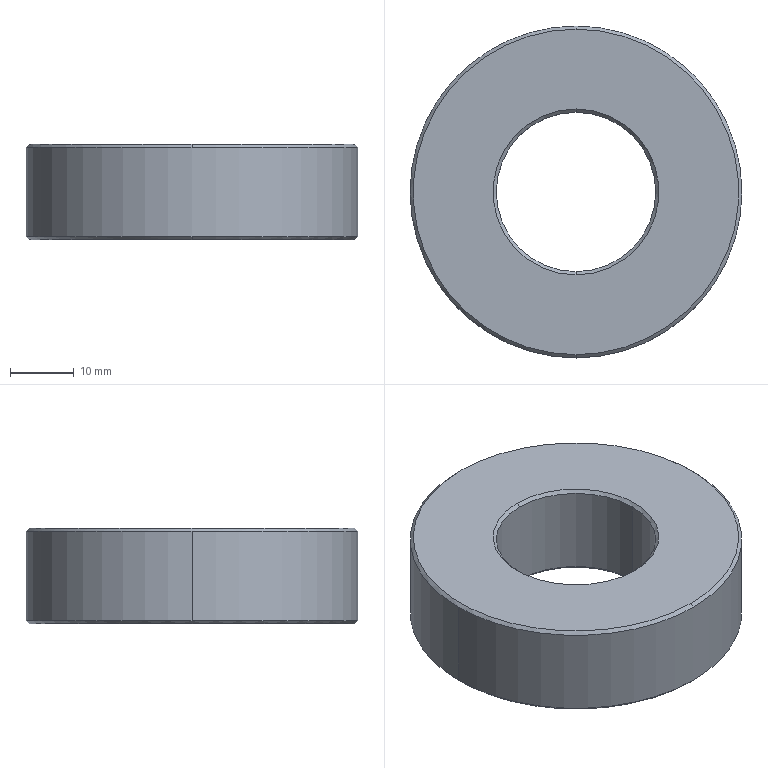Part | 1 solid | 14 faces | box 52 x 52 x 15 mm | volume 24432 mm3 | cone 8 | cylinder 4 | plane 2 | commonest cylinder face diameters 25 x2 52 x2
STEP:
#1=CARTESIAN_POINT('',(0.,-25.5,-7.5));
#2=VERTEX_POINT('',#1);
#3=CARTESIAN_POINT('',(0.,25.5,-7.5));
#4=VERTEX_POINT('',#3);
#5=CARTESIAN_POINT('',(0.,0.,-7.5));
#6=DIRECTION('',(0.,0.,1.));
#7=DIRECTION('',(0.,-1.,0.));
#8=AXIS2_PLACEMENT_3D('',#5,#6,#7);
#9=CIRCLE('',#8,25.5);
#10=EDGE_CURVE('',#2,#4,#9,.T.);
#11=ORIENTED_EDGE('',*,*,#10,.T.);
#12=CARTESIAN_POINT('',(0.,26.,-7.));
#13=VERTEX_POINT('',#12);
#14=CARTESIAN_POINT('',(0.,26.,-7.));
#15=DIRECTION('',(0.,0.7071,0.7071));
#16=VECTOR('',#15,1000.);
#17=LINE('',#14,#16);
#18=EDGE_CURVE('',#4,#13,#17,.T.);
#19=ORIENTED_EDGE('',*,*,#18,.T.);
#20=CARTESIAN_POINT('',(26.,0.,-7.));
#21=VERTEX_POINT('',#20);
#22=CARTESIAN_POINT('',(0.,0.,-7.));
#23=DIRECTION('',(0.,0.,-1.));
#24=DIRECTION('',(1.,0.,0.));
#25=AXIS2_PLACEMENT_3D('',#22,#23,#24);
#26=CIRCLE('',#25,26.);
#27=EDGE_CURVE('',#13,#21,#26,.T.);
#28=ORIENTED_EDGE('',*,*,#27,.T.);
#29=CARTESIAN_POINT('',(0.,-26.,-7.));
#30=VERTEX_POINT('',#29);
#31=CARTESIAN_POINT('',(0.,0.,-7.));
#32=DIRECTION('',(0.,0.,-1.));
#33=DIRECTION('',(1.,0.,0.));
#34=AXIS2_PLACEMENT_3D('',#31,#32,#33);
#35=CIRCLE('',#34,26.);
#36=EDGE_CURVE('',#21,#30,#35,.T.);
#37=ORIENTED_EDGE('',*,*,#36,.T.);
#38=CARTESIAN_POINT('',(0.,-26.,-7.));
#39=DIRECTION('',(0.,-0.7071,0.7071));
#40=VECTOR('',#39,1000.);
#41=LINE('',#38,#40);
#42=EDGE_CURVE('',#2,#30,#41,.T.);
#43=ORIENTED_EDGE('',*,*,#42,.F.);
#44=EDGE_LOOP('',(#11,#19,#28,#37,#43));
#45=FACE_OUTER_BOUND('',#44,.T.);
#46=CARTESIAN_POINT('',(0.,0.,-7.));
#47=DIRECTION('',(0.,0.,1.));
#48=DIRECTION('',(0.,-1.,0.));
#49=AXIS2_PLACEMENT_3D('',#46,#47,#48);
#50=CONICAL_SURFACE('',#49,26.,0.7854);
#51=ADVANCED_FACE('',(#45),#50,.T.);
#52=CARTESIAN_POINT('',(0.,-12.5,-7.));
#53=VERTEX_POINT('',#52);
#54=CARTESIAN_POINT('',(-12.5,0.,-7.));
#55=VERTEX_POINT('',#54);
#56=CARTESIAN_POINT('',(0.,0.,-7.));
#57=DIRECTION('',(0.,0.,-1.));
#58=DIRECTION('',(-1.,0.,0.));
#59=AXIS2_PLACEMENT_3D('',#56,#57,#58);
#60=CIRCLE('',#59,12.5);
#61=EDGE_CURVE('',#53,#55,#60,.T.);
#62=ORIENTED_EDGE('',*,*,#61,.F.);
#63=CARTESIAN_POINT('',(0.,-13.,-7.5));
#64=VERTEX_POINT('',#63);
#65=CARTESIAN_POINT('',(0.,-13.,-7.5));
#66=DIRECTION('',(0.,-0.7071,-0.7071));
#67=VECTOR('',#66,1000.);
#68=LINE('',#65,#67);
#69=EDGE_CURVE('',#53,#64,#68,.T.);
#70=ORIENTED_EDGE('',*,*,#69,.T.);
#71=CARTESIAN_POINT('',(0.,13.,-7.5));
#72=VERTEX_POINT('',#71);
#73=CARTESIAN_POINT('',(0.,0.,-7.5));
#74=DIRECTION('',(0.,0.,-1.));
#75=DIRECTION('',(0.,1.,0.));
#76=AXIS2_PLACEMENT_3D('',#73,#74,#75);
#77=CIRCLE('',#76,13.);
#78=EDGE_CURVE('',#64,#72,#77,.T.);
#79=ORIENTED_EDGE('',*,*,#78,.T.);
#80=CARTESIAN_POINT('',(0.,12.5,-7.));
#81=VERTEX_POINT('',#80);
#82=CARTESIAN_POINT('',(0.,13.,-7.5));
#83=DIRECTION('',(0.,0.7071,-0.7071));
#84=VECTOR('',#83,1000.);
#85=LINE('',#82,#84);
#86=EDGE_CURVE('',#81,#72,#85,.T.);
#87=ORIENTED_EDGE('',*,*,#86,.F.);
#88=CARTESIAN_POINT('',(0.,0.,-7.));
#89=DIRECTION('',(0.,0.,-1.));
#90=DIRECTION('',(-1.,0.,0.));
#91=AXIS2_PLACEMENT_3D('',#88,#89,#90);
#92=CIRCLE('',#91,12.5);
#93=EDGE_CURVE('',#55,#81,#92,.T.);
#94=ORIENTED_EDGE('',*,*,#93,.F.);
#95=EDGE_LOOP('',(#62,#70,#79,#87,#94));
#96=FACE_OUTER_BOUND('',#95,.T.);
#97=CARTESIAN_POINT('',(0.,0.,-7.5));
#98=DIRECTION('',(0.,0.,-1.));
#99=DIRECTION('',(0.,1.,0.));
#100=AXIS2_PLACEMENT_3D('',#97,#98,#99);
#101=CONICAL_SURFACE('',#100,13.,0.7854);
#102=ADVANCED_FACE('',(#96),#101,.F.);
#103=CARTESIAN_POINT('',(0.,26.,7.));
#104=VERTEX_POINT('',#103);
#105=CARTESIAN_POINT('',(26.,0.,7.));
#106=VERTEX_POINT('',#105);
#107=CARTESIAN_POINT('',(0.,0.,7.));
#108=DIRECTION('',(0.,0.,-1.));
#109=DIRECTION('',(-1.,0.,0.));
#110=AXIS2_PLACEMENT_3D('',#107,#108,#109);
#111=CIRCLE('',#110,26.);
#112=EDGE_CURVE('',#104,#106,#111,.T.);
#113=ORIENTED_EDGE('',*,*,#112,.T.);
#114=CARTESIAN_POINT('',(26.,0.,7.5));
#115=DIRECTION('',(0.,0.,-1.));
#116=VECTOR('',#115,1000.);
#117=LINE('',#114,#116);
#118=EDGE_CURVE('',#106,#21,#117,.T.);
#119=ORIENTED_EDGE('',*,*,#118,.T.);
#120=ORIENTED_EDGE('',*,*,#27,.F.);
#121=CARTESIAN_POINT('',(-26.,0.,-7.));
#122=VERTEX_POINT('',#121);
#123=CARTESIAN_POINT('',(0.,0.,-7.));
#124=DIRECTION('',(0.,0.,-1.));
#125=DIRECTION('',(1.,0.,0.));
#126=AXIS2_PLACEMENT_3D('',#123,#124,#125);
#127=CIRCLE('',#126,26.);
#128=EDGE_CURVE('',#122,#13,#127,.T.);
#129=ORIENTED_EDGE('',*,*,#128,.F.);
#130=CARTESIAN_POINT('',(-26.,0.,7.));
#131=VERTEX_POINT('',#130);
#132=CARTESIAN_POINT('',(-26.,0.,7.5));
#133=DIRECTION('',(0.,0.,-1.));
#134=VECTOR('',#133,1000.);
#135=LINE('',#132,#134);
#136=EDGE_CURVE('',#131,#122,#135,.T.);
#137=ORIENTED_EDGE('',*,*,#136,.F.);
#138=CARTESIAN_POINT('',(0.,0.,7.));
#139=DIRECTION('',(0.,0.,-1.));
#140=DIRECTION('',(-1.,0.,0.));
#141=AXIS2_PLACEMENT_3D('',#138,#139,#140);
#142=CIRCLE('',#141,26.);
#143=EDGE_CURVE('',#131,#104,#142,.T.);
#144=ORIENTED_EDGE('',*,*,#143,.T.);
#145=EDGE_LOOP('',(#113,#119,#120,#129,#137,#144));
#146=FACE_OUTER_BOUND('',#145,.T.);
#147=CARTESIAN_POINT('',(0.,0.,7.5));
#148=DIRECTION('',(0.,0.,-1.));
#149=DIRECTION('',(-1.,0.,0.));
#150=AXIS2_PLACEMENT_3D('',#147,#148,#149);
#151=CYLINDRICAL_SURFACE('',#150,26.);
#152=ADVANCED_FACE('',(#146),#151,.T.);
#153=CARTESIAN_POINT('',(12.5,0.,7.));
#154=VERTEX_POINT('',#153);
#155=CARTESIAN_POINT('',(0.,-12.5,7.));
#156=VERTEX_POINT('',#155);
#157=CARTESIAN_POINT('',(0.,0.,7.));
#158=DIRECTION('',(0.,0.,-1.));
#159=DIRECTION('',(-1.,0.,0.));
#160=AXIS2_PLACEMENT_3D('',#157,#158,#159);
#161=CIRCLE('',#160,12.5);
#162=EDGE_CURVE('',#154,#156,#161,.T.);
#163=ORIENTED_EDGE('',*,*,#162,.F.);
#164=CARTESIAN_POINT('',(12.5,0.,-7.));
#165=VERTEX_POINT('',#164);
#166=CARTESIAN_POINT('',(12.5,0.,7.5));
#167=DIRECTION('',(0.,0.,-1.));
#168=VECTOR('',#167,1000.);
#169=LINE('',#166,#168);
#170=EDGE_CURVE('',#154,#165,#169,.T.);
#171=ORIENTED_EDGE('',*,*,#170,.T.);
#172=CARTESIAN_POINT('',(0.,0.,-7.));
#173=DIRECTION('',(0.,0.,-1.));
#174=DIRECTION('',(-1.,0.,0.));
#175=AXIS2_PLACEMENT_3D('',#172,#173,#174);
#176=CIRCLE('',#175,12.5);
#177=EDGE_CURVE('',#165,#53,#176,.T.);
#178=ORIENTED_EDGE('',*,*,#177,.T.);
#179=ORIENTED_EDGE('',*,*,#61,.T.);
#180=CARTESIAN_POINT('',(-12.5,0.,7.));
#181=VERTEX_POINT('',#180);
#182=CARTESIAN_POINT('',(-12.5,0.,7.5));
#183=DIRECTION('',(0.,0.,-1.));
#184=VECTOR('',#183,1000.);
#185=LINE('',#182,#184);
#186=EDGE_CURVE('',#181,#55,#185,.T.);
#187=ORIENTED_EDGE('',*,*,#186,.F.);
#188=CARTESIAN_POINT('',(0.,0.,7.));
#189=DIRECTION('',(0.,0.,-1.));
#190=DIRECTION('',(-1.,0.,0.));
#191=AXIS2_PLACEMENT_3D('',#188,#189,#190);
#192=CIRCLE('',#191,12.5);
#193=EDGE_CURVE('',#156,#181,#192,.T.);
#194=ORIENTED_EDGE('',*,*,#193,.F.);
#195=EDGE_LOOP('',(#163,#171,#178,#179,#187,#194));
#196=FACE_OUTER_BOUND('',#195,.T.);
#197=CARTESIAN_POINT('',(0.,0.,7.5));
#198=DIRECTION('',(0.,0.,-1.));
#199=DIRECTION('',(-1.,0.,0.));
#200=AXIS2_PLACEMENT_3D('',#197,#198,#199);
#201=CYLINDRICAL_SURFACE('',#200,12.5);
#202=ADVANCED_FACE('',(#196),#201,.F.);
#203=CARTESIAN_POINT('',(0.,25.5,7.5));
#204=VERTEX_POINT('',#203);
#205=CARTESIAN_POINT('',(0.,-25.5,7.5));
#206=VERTEX_POINT('',#205);
#207=CARTESIAN_POINT('',(0.,0.,7.5));
#208=DIRECTION('',(0.,0.,-1.));
#209=DIRECTION('',(0.,1.,0.));
#210=AXIS2_PLACEMENT_3D('',#207,#208,#209);
#211=CIRCLE('',#210,25.5);
#212=EDGE_CURVE('',#204,#206,#211,.T.);
#213=ORIENTED_EDGE('',*,*,#212,.T.);
#214=CARTESIAN_POINT('',(0.,-26.,7.));
#215=VERTEX_POINT('',#214);
#216=CARTESIAN_POINT('',(0.,-26.,7.));
#217=DIRECTION('',(0.,-0.7071,-0.7071));
#218=VECTOR('',#217,1000.);
#219=LINE('',#216,#218);
#220=EDGE_CURVE('',#206,#215,#219,.T.);
#221=ORIENTED_EDGE('',*,*,#220,.T.);
#222=CARTESIAN_POINT('',(0.,0.,7.));
#223=DIRECTION('',(0.,0.,-1.));
#224=DIRECTION('',(-1.,0.,0.));
#225=AXIS2_PLACEMENT_3D('',#222,#223,#224);
#226=CIRCLE('',#225,26.);
#227=EDGE_CURVE('',#106,#215,#226,.T.);
#228=ORIENTED_EDGE('',*,*,#227,.F.);
#229=ORIENTED_EDGE('',*,*,#112,.F.);
#230=CARTESIAN_POINT('',(0.,26.,7.));
#231=DIRECTION('',(0.,0.7071,-0.7071));
#232=VECTOR('',#231,1000.);
#233=LINE('',#230,#232);
#234=EDGE_CURVE('',#204,#104,#233,.T.);
#235=ORIENTED_EDGE('',*,*,#234,.F.);
#236=EDGE_LOOP('',(#213,#221,#228,#229,#235));
#237=FACE_OUTER_BOUND('',#236,.T.);
#238=CARTESIAN_POINT('',(0.,0.,7.));
#239=DIRECTION('',(0.,0.,-1.));
#240=DIRECTION('',(0.,1.,0.));
#241=AXIS2_PLACEMENT_3D('',#238,#239,#240);
#242=CONICAL_SURFACE('',#241,26.,0.7854);
#243=ADVANCED_FACE('',(#237),#242,.T.);
#244=ORIENTED_EDGE('',*,*,#193,.T.);
#245=CARTESIAN_POINT('',(0.,12.5,7.));
#246=VERTEX_POINT('',#245);
#247=CARTESIAN_POINT('',(0.,0.,7.));
#248=DIRECTION('',(0.,0.,-1.));
#249=DIRECTION('',(-1.,0.,0.));
#250=AXIS2_PLACEMENT_3D('',#247,#248,#249);
#251=CIRCLE('',#250,12.5);
#252=EDGE_CURVE('',#181,#246,#251,.T.);
#253=ORIENTED_EDGE('',*,*,#252,.T.);
#254=CARTESIAN_POINT('',(0.,13.,7.5));
#255=VERTEX_POINT('',#254);
#256=CARTESIAN_POINT('',(0.,13.,7.5));
#257=DIRECTION('',(0.,0.7071,0.7071));
#258=VECTOR('',#257,1000.);
#259=LINE('',#256,#258);
#260=EDGE_CURVE('',#246,#255,#259,.T.);
#261=ORIENTED_EDGE('',*,*,#260,.T.);
#262=CARTESIAN_POINT('',(0.,-13.,7.5));
#263=VERTEX_POINT('',#262);
#264=CARTESIAN_POINT('',(0.,0.,7.5));
#265=DIRECTION('',(0.,0.,-1.));
#266=DIRECTION('',(0.,-1.,0.));
#267=AXIS2_PLACEMENT_3D('',#264,#265,#266);
#268=CIRCLE('',#267,13.);
#269=EDGE_CURVE('',#263,#255,#268,.T.);
#270=ORIENTED_EDGE('',*,*,#269,.F.);
#271=CARTESIAN_POINT('',(0.,-13.,7.5));
#272=DIRECTION('',(0.,-0.7071,0.7071));
#273=VECTOR('',#272,1000.);
#274=LINE('',#271,#273);
#275=EDGE_CURVE('',#156,#263,#274,.T.);
#276=ORIENTED_EDGE('',*,*,#275,.F.);
#277=EDGE_LOOP('',(#244,#253,#261,#270,#276));
#278=FACE_OUTER_BOUND('',#277,.T.);
#279=CARTESIAN_POINT('',(0.,0.,7.5));
#280=DIRECTION('',(0.,0.,1.));
#281=DIRECTION('',(0.,-1.,0.));
#282=AXIS2_PLACEMENT_3D('',#279,#280,#281);
#283=CONICAL_SURFACE('',#282,13.,0.7854);
#284=ADVANCED_FACE('',(#278),#283,.F.);
#285=ORIENTED_EDGE('',*,*,#10,.F.);
#286=CARTESIAN_POINT('',(0.,0.,-7.5));
#287=DIRECTION('',(0.,0.,1.));
#288=DIRECTION('',(0.,-1.,0.));
#289=AXIS2_PLACEMENT_3D('',#286,#287,#288);
#290=CIRCLE('',#289,25.5);
#291=EDGE_CURVE('',#4,#2,#290,.T.);
#292=ORIENTED_EDGE('',*,*,#291,.F.);
#293=EDGE_LOOP('',(#285,#292));
#294=FACE_OUTER_BOUND('',#293,.T.);
#295=CARTESIAN_POINT('',(0.,0.,-7.5));
#296=DIRECTION('',(0.,0.,-1.));
#297=DIRECTION('',(0.,1.,0.));
#298=AXIS2_PLACEMENT_3D('',#295,#296,#297);
#299=CIRCLE('',#298,13.);
#300=EDGE_CURVE('',#72,#64,#299,.T.);
#301=ORIENTED_EDGE('',*,*,#300,.F.);
#302=ORIENTED_EDGE('',*,*,#78,.F.);
#303=EDGE_LOOP('',(#301,#302));
#304=FACE_BOUND('',#303,.T.);
#305=CARTESIAN_POINT('',(0.,0.,-7.5));
#306=DIRECTION('',(0.,0.,1.));
#307=DIRECTION('',(1.,0.,0.));
#308=AXIS2_PLACEMENT_3D('',#305,#306,#307);
#309=PLANE('',#308);
#310=ADVANCED_FACE('',(#294,#304),#309,.F.);
#311=ORIENTED_EDGE('',*,*,#18,.F.);
#312=ORIENTED_EDGE('',*,*,#291,.T.);
#313=ORIENTED_EDGE('',*,*,#42,.T.);
#314=CARTESIAN_POINT('',(0.,0.,-7.));
#315=DIRECTION('',(0.,0.,-1.));
#316=DIRECTION('',(1.,0.,0.));
#317=AXIS2_PLACEMENT_3D('',#314,#315,#316);
#318=CIRCLE('',#317,26.);
#319=EDGE_CURVE('',#30,#122,#318,.T.);
#320=ORIENTED_EDGE('',*,*,#319,.T.);
#321=ORIENTED_EDGE('',*,*,#128,.T.);
#322=EDGE_LOOP('',(#311,#312,#313,#320,#321));
#323=FACE_OUTER_BOUND('',#322,.T.);
#324=CARTESIAN_POINT('',(0.,0.,-7.));
#325=DIRECTION('',(0.,0.,1.));
#326=DIRECTION('',(0.,-1.,0.));
#327=AXIS2_PLACEMENT_3D('',#324,#325,#326);
#328=CONICAL_SURFACE('',#327,26.,0.7854);
#329=ADVANCED_FACE('',(#323),#328,.T.);
#330=ORIENTED_EDGE('',*,*,#69,.F.);
#331=ORIENTED_EDGE('',*,*,#177,.F.);
#332=CARTESIAN_POINT('',(0.,0.,-7.));
#333=DIRECTION('',(0.,0.,-1.));
#334=DIRECTION('',(-1.,0.,0.));
#335=AXIS2_PLACEMENT_3D('',#332,#333,#334);
#336=CIRCLE('',#335,12.5);
#337=EDGE_CURVE('',#81,#165,#336,.T.);
#338=ORIENTED_EDGE('',*,*,#337,.F.);
#339=ORIENTED_EDGE('',*,*,#86,.T.);
#340=ORIENTED_EDGE('',*,*,#300,.T.);
#341=EDGE_LOOP('',(#330,#331,#338,#339,#340));
#342=FACE_OUTER_BOUND('',#341,.T.);
#343=CARTESIAN_POINT('',(0.,0.,-7.5));
#344=DIRECTION('',(0.,0.,-1.));
#345=DIRECTION('',(0.,1.,0.));
#346=AXIS2_PLACEMENT_3D('',#343,#344,#345);
#347=CONICAL_SURFACE('',#346,13.,0.7854);
#348=ADVANCED_FACE('',(#342),#347,.F.);
#349=ORIENTED_EDGE('',*,*,#118,.F.);
#350=ORIENTED_EDGE('',*,*,#227,.T.);
#351=CARTESIAN_POINT('',(0.,0.,7.));
#352=DIRECTION('',(0.,0.,-1.));
#353=DIRECTION('',(-1.,0.,0.));
#354=AXIS2_PLACEMENT_3D('',#351,#352,#353);
#355=CIRCLE('',#354,26.);
#356=EDGE_CURVE('',#215,#131,#355,.T.);
#357=ORIENTED_EDGE('',*,*,#356,.T.);
#358=ORIENTED_EDGE('',*,*,#136,.T.);
#359=ORIENTED_EDGE('',*,*,#319,.F.);
#360=ORIENTED_EDGE('',*,*,#36,.F.);
#361=EDGE_LOOP('',(#349,#350,#357,#358,#359,#360));
#362=FACE_OUTER_BOUND('',#361,.T.);
#363=CARTESIAN_POINT('',(0.,0.,7.5));
#364=DIRECTION('',(0.,0.,-1.));
#365=DIRECTION('',(-1.,0.,0.));
#366=AXIS2_PLACEMENT_3D('',#363,#364,#365);
#367=CYLINDRICAL_SURFACE('',#366,26.);
#368=ADVANCED_FACE('',(#362),#367,.T.);
#369=ORIENTED_EDGE('',*,*,#170,.F.);
#370=CARTESIAN_POINT('',(0.,0.,7.));
#371=DIRECTION('',(0.,0.,-1.));
#372=DIRECTION('',(-1.,0.,0.));
#373=AXIS2_PLACEMENT_3D('',#370,#371,#372);
#374=CIRCLE('',#373,12.5);
#375=EDGE_CURVE('',#246,#154,#374,.T.);
#376=ORIENTED_EDGE('',*,*,#375,.F.);
#377=ORIENTED_EDGE('',*,*,#252,.F.);
#378=ORIENTED_EDGE('',*,*,#186,.T.);
#379=ORIENTED_EDGE('',*,*,#93,.T.);
#380=ORIENTED_EDGE('',*,*,#337,.T.);
#381=EDGE_LOOP('',(#369,#376,#377,#378,#379,#380));
#382=FACE_OUTER_BOUND('',#381,.T.);
#383=CARTESIAN_POINT('',(0.,0.,7.5));
#384=DIRECTION('',(0.,0.,-1.));
#385=DIRECTION('',(-1.,0.,0.));
#386=AXIS2_PLACEMENT_3D('',#383,#384,#385);
#387=CYLINDRICAL_SURFACE('',#386,12.5);
#388=ADVANCED_FACE('',(#382),#387,.F.);
#389=ORIENTED_EDGE('',*,*,#220,.F.);
#390=CARTESIAN_POINT('',(0.,0.,7.5));
#391=DIRECTION('',(0.,0.,-1.));
#392=DIRECTION('',(0.,1.,0.));
#393=AXIS2_PLACEMENT_3D('',#390,#391,#392);
#394=CIRCLE('',#393,25.5);
#395=EDGE_CURVE('',#206,#204,#394,.T.);
#396=ORIENTED_EDGE('',*,*,#395,.T.);
#397=ORIENTED_EDGE('',*,*,#234,.T.);
#398=ORIENTED_EDGE('',*,*,#143,.F.);
#399=ORIENTED_EDGE('',*,*,#356,.F.);
#400=EDGE_LOOP('',(#389,#396,#397,#398,#399));
#401=FACE_OUTER_BOUND('',#400,.T.);
#402=CARTESIAN_POINT('',(0.,0.,7.));
#403=DIRECTION('',(0.,0.,-1.));
#404=DIRECTION('',(0.,1.,0.));
#405=AXIS2_PLACEMENT_3D('',#402,#403,#404);
#406=CONICAL_SURFACE('',#405,26.,0.7854);
#407=ADVANCED_FACE('',(#401),#406,.T.);
#408=ORIENTED_EDGE('',*,*,#260,.F.);
#409=ORIENTED_EDGE('',*,*,#375,.T.);
#410=ORIENTED_EDGE('',*,*,#162,.T.);
#411=ORIENTED_EDGE('',*,*,#275,.T.);
#412=CARTESIAN_POINT('',(0.,0.,7.5));
#413=DIRECTION('',(0.,0.,-1.));
#414=DIRECTION('',(0.,-1.,0.));
#415=AXIS2_PLACEMENT_3D('',#412,#413,#414);
#416=CIRCLE('',#415,13.);
#417=EDGE_CURVE('',#255,#263,#416,.T.);
#418=ORIENTED_EDGE('',*,*,#417,.F.);
#419=EDGE_LOOP('',(#408,#409,#410,#411,#418));
#420=FACE_OUTER_BOUND('',#419,.T.);
#421=CARTESIAN_POINT('',(0.,0.,7.5));
#422=DIRECTION('',(0.,0.,1.));
#423=DIRECTION('',(0.,-1.,0.));
#424=AXIS2_PLACEMENT_3D('',#421,#422,#423);
#425=CONICAL_SURFACE('',#424,13.,0.7854);
#426=ADVANCED_FACE('',(#420),#425,.F.);
#427=ORIENTED_EDGE('',*,*,#212,.F.);
#428=ORIENTED_EDGE('',*,*,#395,.F.);
#429=EDGE_LOOP('',(#427,#428));
#430=FACE_OUTER_BOUND('',#429,.T.);
#431=ORIENTED_EDGE('',*,*,#269,.T.);
#432=ORIENTED_EDGE('',*,*,#417,.T.);
#433=EDGE_LOOP('',(#431,#432));
#434=FACE_BOUND('',#433,.T.);
#435=CARTESIAN_POINT('',(0.,0.,7.5));
#436=DIRECTION('',(0.,0.,1.));
#437=DIRECTION('',(1.,0.,0.));
#438=AXIS2_PLACEMENT_3D('',#435,#436,#437);
#439=PLANE('',#438);
#440=ADVANCED_FACE('',(#430,#434),#439,.T.);
#441=CLOSED_SHELL('',(#51,#102,#152,#202,#243,#284,#310,#329,#348,#368,#388,#407,#426,#440));
#442=MANIFOLD_SOLID_BREP('',#441);
#443=CARTESIAN_POINT('',(0.,0.,0.));
#444=DIRECTION('',(0.,0.,1.));
#445=DIRECTION('',(1.,0.,0.));
#446=AXIS2_PLACEMENT_3D('',#443,#444,#445);
#447=(LENGTH_UNIT()NAMED_UNIT(*)SI_UNIT(.MILLI.,.METRE.));
#448=UNCERTAINTY_MEASURE_WITH_UNIT(LENGTH_MEASURE(0.00001),#447,'','');
#449=(NAMED_UNIT(*)PLANE_ANGLE_UNIT()SI_UNIT($,.RADIAN.));
#450=(NAMED_UNIT(*)SI_UNIT($,.STERADIAN.)SOLID_ANGLE_UNIT());
#451=(GEOMETRIC_REPRESENTATION_CONTEXT(3)GLOBAL_UNCERTAINTY_ASSIGNED_CONTEXT((#448))GLOBAL_UNIT_ASSIGNED_CONTEXT((#447,#449,#450))REPRESENTATION_CONTEXT('',''));
#452=ADVANCED_BREP_SHAPE_REPRESENTATION('',(#442,#446),#451);